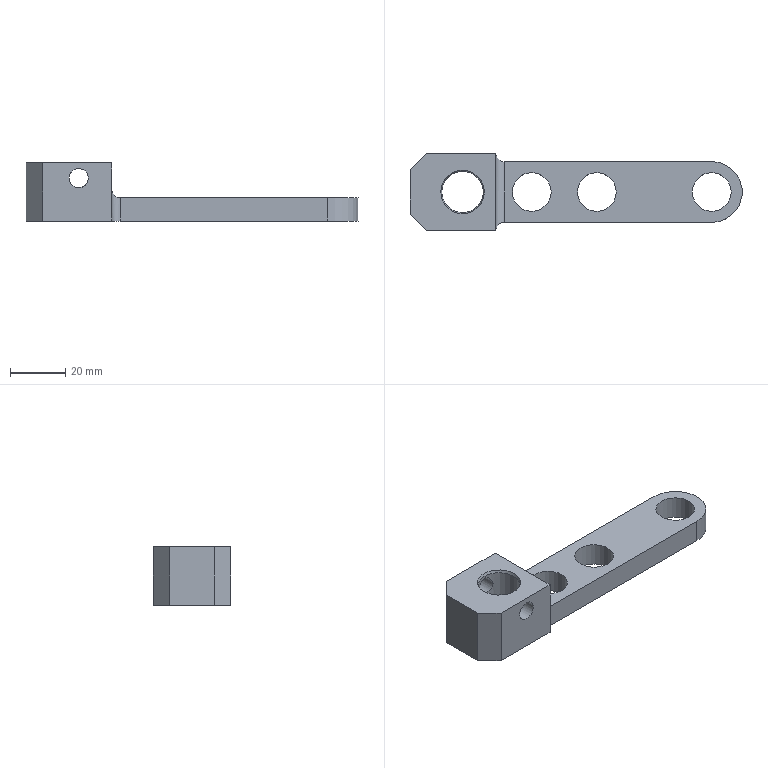NC program | NX | posted with a generic post | part box 120 x 28 x 21 mm
Whole program:
N10 G17 G21 G94 G90
(DRILLING_3 , TOOL : 倒角D6-90度)
N12 T03 M6
N14 G54
N16 G17 G0 G90 X-19.008 Y-15.5 B0. C0. S1200 M3
N18 G43 Z20. H3
N20 G94 G81 G99 Z-1. B-180. C-180. F60. R3.
N22 G80
N24 G0 X-19.008 Y-15.5 Z20.
N26 M5
(DRILLING_4 , TOOL : 钻头D6.8-73-105)
N28 T09 M6
N30 G54
N32 G17 G0 G90 X-19.008 Y-15.5 B0. C0. S800 M3
N34 G43 Z20. H9
N36 G94 G81 G99 Z-10. B-180. C-180. F60. R3.
N38 G80
N40 G0 X-19.008 Y-15.5 Z20.
N42 M5
(PLANAR_MILL_5_COPY_COPY , TOOL : 倒角D6-90度)
N44 T03 M6
N46 G54
N48 G17 G0 G90 X-18.742 Y-14.432 B0. C0. S3000 M3
N50 G43 Z20. H3
N52 Z0. B-180. C-180.
N54 G94 G1 Z-2. F60.
N56 G41 X-18.708 Y-14.235 D3
N58 Y-14.2
N60 G3 X-19.008 Y-13.9 R0.3
N62 X-20.608 Y-15.5 R1.6
N64 X-19.008 Y-13.9 R-1.6
N66 X-19.308 Y-14.2 R0.3
N68 G1 Y-14.235
N70 G40
N72 X-19.273 Y-14.432
N74 Z0.
N76 G0 Z20.
N78 M5
(PLANAR_MILL_5 , TOOL : D6-18-D6-50-3T-精)
N80 T06 M6
N82 G54
N84 G17 G0 G90 X-18.929 Y-15.478 B0. C0. S3000 M3
N86 G43 Z20. H6
N88 Z-7. B-180. C-180.
N90 G94 G1 Z-9. F60.
N92 G41 X-18.708 Y-15.418 D6
N94 G3 X-19.008 Y-15.118 R0.3
N96 X-19.39 Y-15.5 R0.382
N98 X-19.008 Y-15.118 R-0.382
N100 X-19.308 Y-15.418 R0.3
N102 G40
N104 G1 X-19.29 Y-15.516
N106 X-18.725 Y-15.51
N108 G41 X-18.708 Y-15.412
N110 G3 X-19.008 Y-15.112 R0.3
N112 X-19.396 Y-15.5 R0.388
N114 X-19.008 Y-15.112 R-0.388
N116 X-19.308 Y-15.412 R0.3
N118 G40
N120 G1 X-19.29 Y-15.51
N122 X-18.725 Y-15.504
N124 G41 X-18.708 Y-15.406
N126 G3 X-19.008 Y-15.106 R0.3
N128 X-19.402 Y-15.5 R0.394
N130 X-19.008 Y-15.106 R-0.394
N132 X-19.308 Y-15.406 R0.3
N134 G40
N136 G1 X-19.29 Y-15.504
N138 X-18.725 Y-15.498
N140 G41 X-18.708 Y-15.4
N142 G3 X-19.008 Y-15.1 R0.3
N144 X-19.408 Y-15.5 R0.4
N146 X-19.008 Y-15.1 R-0.4
N148 X-19.308 Y-15.4 R0.3
N150 G40
N152 G1 X-19.103 Y-15.468
N154 Z-7.
N156 G0 Z20.
(PLANAR_MILL_5_COPY , TOOL : D6-18-D6-50-3T-精)
N158 X-19.024 Y-15.469
N160 Z-7.
N162 G1 Z-9. F30.
N164 G41 X-18.841 Y-15.389
N166 X-18.708 Y-15.3
N168 G3 X-19.008 Y-15. R0.3
N170 X-19.508 Y-15.5 R0.5
N172 X-19.008 Y-15. R-0.5
N174 X-19.308 Y-15.3 R0.3
N176 G40
N178 G1 X-19.273 Y-15.497
N180 X-18.742
N182 G41 X-18.708 Y-15.3
N184 G3 X-19.008 Y-15. R0.3
N186 X-19.508 Y-15.5 R0.5
N188 X-19.008 Y-15. R-0.5
N190 X-19.308 Y-15.3 R0.3
N192 G40
N194 G1 X-19.273 Y-15.497
N196 X-18.742
N198 G41 X-18.708 Y-15.3
N200 G3 X-19.008 Y-15. R0.3
N202 X-19.508 Y-15.5 R0.5
N204 X-19.008 Y-15. R-0.5
N206 X-19.308 Y-15.3 R0.3
N208 G1 X-19.174 Y-15.389
N210 G40
N212 X-18.991 Y-15.469
N214 Z-7.
N216 G0 Z20.
N218 M5
N220 M2